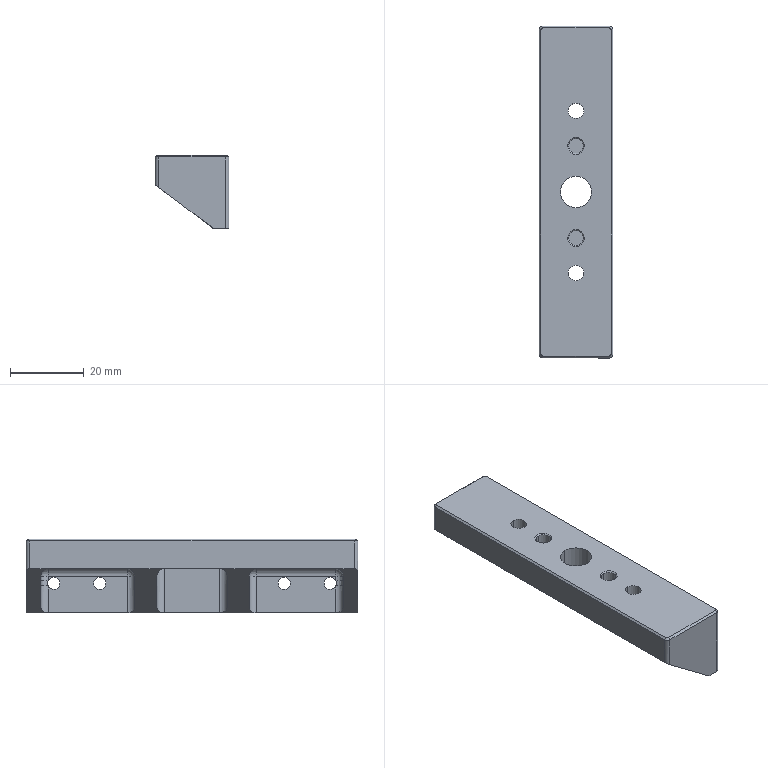Part | 1 solid | 90 faces | box 20 x 90 x 20 mm | volume 19711 mm3 | cylinder 42 | plane 30 | cone 12 | sphere 4 | spline 2 | commonest cylinder face diameters 4 x24 3.3 x8 2 x4 4.2 x4 8.5 x2